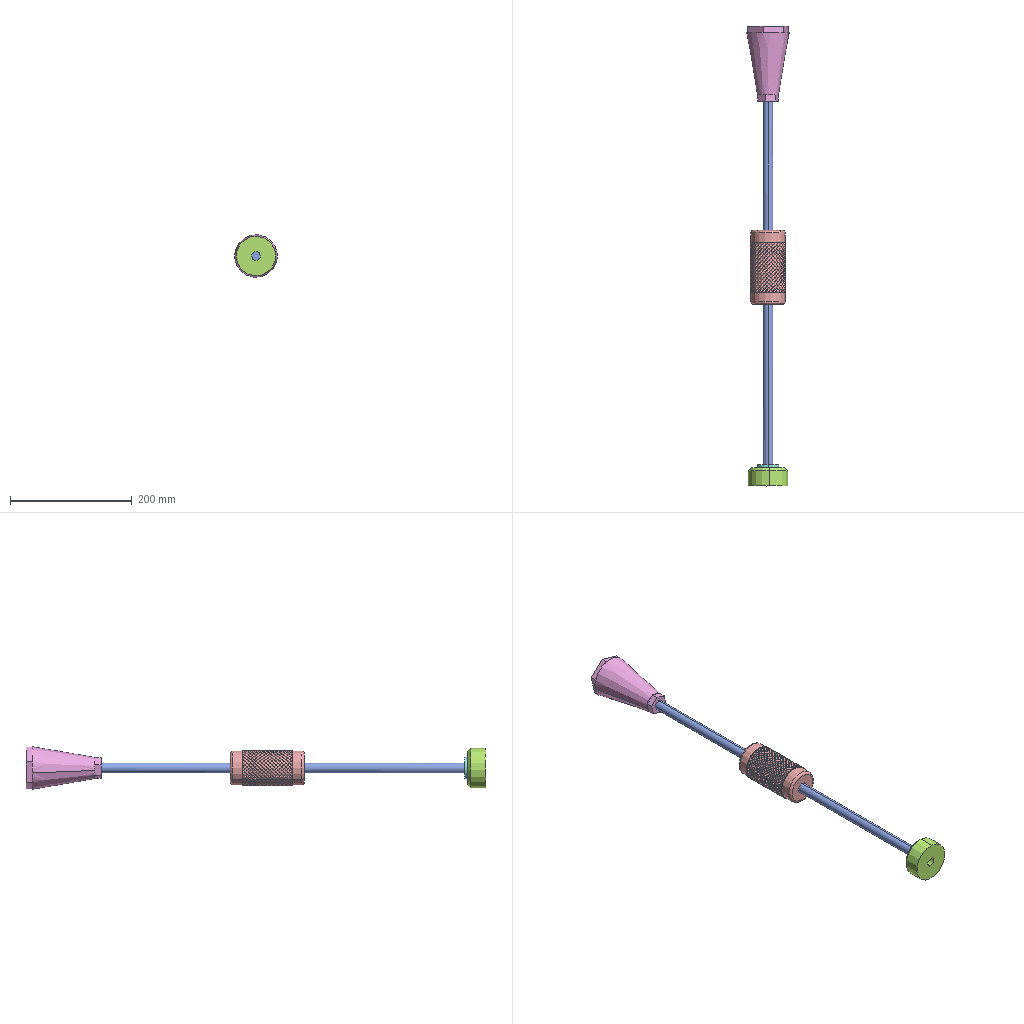Assembly | SolidWorks | 5 different items | 5 placed | box 70 x 754 x 70 mm
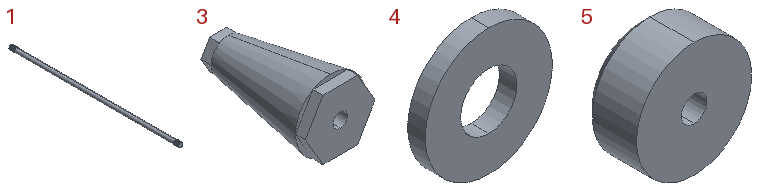Parts list (item | quantity | size | volume | features):
1 | x1 | 16 x 650 x 16 mm | 130458 mm3 | features SweepThread 2, Extrusion 1
2 | x1 | - | - | features Helix 2, ICE 2, SweepCut 2, CirPattern 1, Extrusion 1, Fillet 1
3 | x1 | 70 x 123 x 70 mm | 249186 mm3 | features Extrusion 1, HoleWzd 1, ICE 1, Revolution 1
4 | x1 | 36 x 5 x 36 mm | 4084 mm3 | features Extrusion 1
5 | x1 | 65 x 30 x 65 mm | 92174 mm3 | features Chamfer 1, Extrusion 1, HoleWzd 1
Mates (type | each side: item.copy, entity, surface, feature):
Concentric | 2.1 face cylinder Boss-Extrude1 | 1.1 face cylinder Boss-Extrude1
Coincident | 1.1 plane | assembly plane | 3 times
Concentric | 1.1 face cylinder Boss-Extrude1 | 5.1 face cylinder M16x1.5 Tapped Hole1
Concentric | 1.1 face cylinder Boss-Extrude1 | 3.1 face cone Revolve1
Concentric | 1.1 face cylinder Boss-Extrude1 | 4.1 face cylinder Boss-Extrude1
Coincident | 5.1 face plane Boss-Extrude1 | 4.1 face plane Boss-Extrude1
DistanceDim | 5.1 face plane Boss-Extrude1 | 1.1 face plane Boss-Extrude1